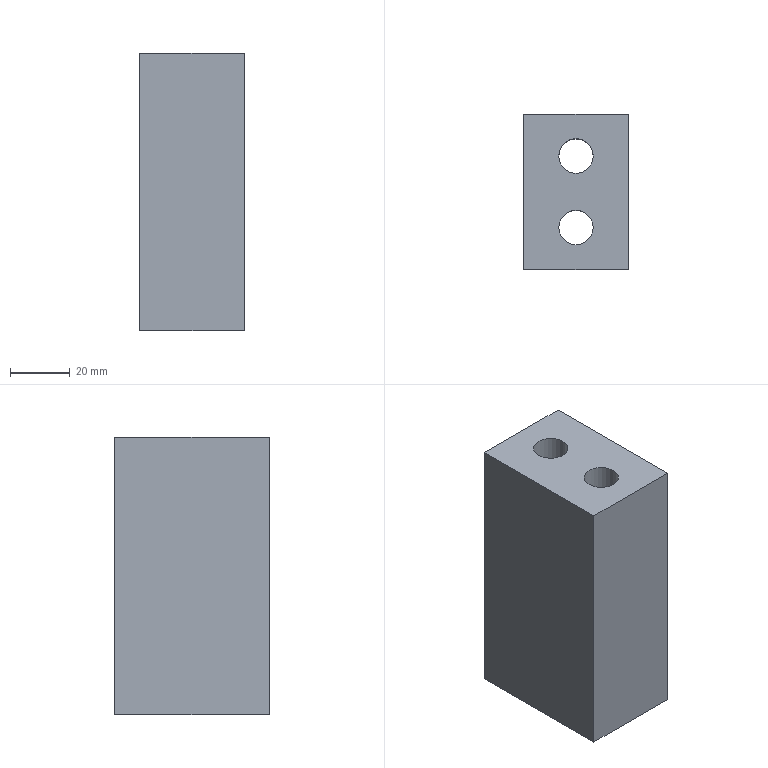Part | NX | features solid 2 | 1 solid | 12 faces | box 35 x 52 x 93 mm | volume 130929 mm3 | plane 8 | cylinder 4 | commonest cylinder face diameters 11.507 x2 18.008 x2
STEP:
#1=CARTESIAN_POINT('',(1828.477,105.595,64.999));
#2=VERTEX_POINT('',#1);
#3=CARTESIAN_POINT('',(1793.477,105.595,64.999));
#4=VERTEX_POINT('',#3);
#5=CARTESIAN_POINT('',(1793.477,105.595,64.999));
#6=DIRECTION('',(1.,0.,-0.000000004));
#7=VECTOR('',#6,1000.);
#8=LINE('',#5,#7);
#9=EDGE_CURVE('',#2,#4,#8,.F.);
#10=ORIENTED_EDGE('',*,*,#9,.F.);
#11=CARTESIAN_POINT('',(1828.477,105.595,-28.001));
#12=VERTEX_POINT('',#11);
#13=CARTESIAN_POINT('',(1828.477,105.595,44.999));
#14=DIRECTION('',(0.000000004,0.,1.));
#15=VECTOR('',#14,1000.);
#16=LINE('',#13,#15);
#17=EDGE_CURVE('',#12,#2,#16,.T.);
#18=ORIENTED_EDGE('',*,*,#17,.F.);
#19=CARTESIAN_POINT('',(1793.477,105.595,-28.001));
#20=VERTEX_POINT('',#19);
#21=CARTESIAN_POINT('',(1793.477,105.595,-28.001));
#22=DIRECTION('',(-1.,0.,0.000000004));
#23=VECTOR('',#22,1000.);
#24=LINE('',#21,#23);
#25=EDGE_CURVE('',#12,#20,#24,.T.);
#26=ORIENTED_EDGE('',*,*,#25,.T.);
#27=CARTESIAN_POINT('',(1793.477,105.595,44.999));
#28=DIRECTION('',(0.000000004,0.,1.));
#29=VECTOR('',#28,1000.);
#30=LINE('',#27,#29);
#31=EDGE_CURVE('',#20,#4,#30,.T.);
#32=ORIENTED_EDGE('',*,*,#31,.T.);
#33=EDGE_LOOP('',(#10,#18,#26,#32));
#34=FACE_BOUND('',#33,.T.);
#35=CARTESIAN_POINT('',(1793.477,105.595,44.999));
#36=DIRECTION('',(0.,-1.,0.));
#37=DIRECTION('',(0.000000004,0.,1.));
#38=AXIS2_PLACEMENT_3D('',#35,#36,#37);
#39=PLANE('',#38);
#40=ADVANCED_FACE('',(#34),#39,.F.);
#41=CARTESIAN_POINT('',(1801.973,91.595,-28.001));
#42=VERTEX_POINT('',#41);
#43=CARTESIAN_POINT('',(1810.977,91.595,-28.001));
#44=DIRECTION('',(0.000000004,0.,1.));
#45=DIRECTION('',(-1.,0.,0.000000004));
#46=AXIS2_PLACEMENT_3D('',#43,#44,#45);
#47=CIRCLE('',#46,9.004);
#48=EDGE_CURVE('',#42,#42,#47,.F.);
#49=ORIENTED_EDGE('',*,*,#48,.F.);
#50=EDGE_LOOP('',(#49));
#51=FACE_BOUND('',#50,.T.);
#52=CARTESIAN_POINT('',(1801.973,67.595,-28.001));
#53=VERTEX_POINT('',#52);
#54=CARTESIAN_POINT('',(1810.977,67.595,-28.001));
#55=DIRECTION('',(0.000000004,0.,1.));
#56=DIRECTION('',(-1.,0.,0.000000004));
#57=AXIS2_PLACEMENT_3D('',#54,#55,#56);
#58=CIRCLE('',#57,9.004);
#59=EDGE_CURVE('',#53,#53,#58,.F.);
#60=ORIENTED_EDGE('',*,*,#59,.F.);
#61=EDGE_LOOP('',(#60));
#62=FACE_BOUND('',#61,.T.);
#63=CARTESIAN_POINT('',(1793.477,53.595,-28.001));
#64=VERTEX_POINT('',#63);
#65=CARTESIAN_POINT('',(1793.477,-114.905,-28.001));
#66=DIRECTION('',(0.,1.,0.));
#67=VECTOR('',#66,1000.);
#68=LINE('',#65,#67);
#69=EDGE_CURVE('',#64,#20,#68,.T.);
#70=ORIENTED_EDGE('',*,*,#69,.T.);
#71=ORIENTED_EDGE('',*,*,#25,.F.);
#72=CARTESIAN_POINT('',(1828.477,53.595,-28.001));
#73=VERTEX_POINT('',#72);
#74=CARTESIAN_POINT('',(1828.477,-114.905,-28.001));
#75=DIRECTION('',(0.,1.,0.));
#76=VECTOR('',#75,1000.);
#77=LINE('',#74,#76);
#78=EDGE_CURVE('',#73,#12,#77,.T.);
#79=ORIENTED_EDGE('',*,*,#78,.F.);
#80=CARTESIAN_POINT('',(1793.477,53.595,-28.001));
#81=DIRECTION('',(-1.,0.,0.000000004));
#82=VECTOR('',#81,1000.);
#83=LINE('',#80,#82);
#84=EDGE_CURVE('',#73,#64,#83,.T.);
#85=ORIENTED_EDGE('',*,*,#84,.T.);
#86=EDGE_LOOP('',(#70,#71,#79,#85));
#87=FACE_BOUND('',#86,.T.);
#88=CARTESIAN_POINT('',(1793.477,-114.905,-28.001));
#89=DIRECTION('',(0.000000004,0.,1.));
#90=DIRECTION('',(0.,1.,0.));
#91=AXIS2_PLACEMENT_3D('',#88,#89,#90);
#92=PLANE('',#91);
#93=ADVANCED_FACE('',(#51,#62,#87),#92,.F.);
#94=CARTESIAN_POINT('',(1805.224,91.595,64.999));
#95=VERTEX_POINT('',#94);
#96=CARTESIAN_POINT('',(1810.977,91.595,64.999));
#97=DIRECTION('',(0.000000004,0.,1.));
#98=DIRECTION('',(-1.,0.,0.000000004));
#99=AXIS2_PLACEMENT_3D('',#96,#97,#98);
#100=CIRCLE('',#99,5.753);
#101=EDGE_CURVE('',#95,#95,#100,.T.);
#102=ORIENTED_EDGE('',*,*,#101,.F.);
#103=EDGE_LOOP('',(#102));
#104=FACE_BOUND('',#103,.T.);
#105=CARTESIAN_POINT('',(1805.224,67.595,64.999));
#106=VERTEX_POINT('',#105);
#107=CARTESIAN_POINT('',(1810.977,67.595,64.999));
#108=DIRECTION('',(0.000000004,0.,1.));
#109=DIRECTION('',(-1.,0.,0.000000004));
#110=AXIS2_PLACEMENT_3D('',#107,#108,#109);
#111=CIRCLE('',#110,5.753);
#112=EDGE_CURVE('',#106,#106,#111,.T.);
#113=ORIENTED_EDGE('',*,*,#112,.F.);
#114=EDGE_LOOP('',(#113));
#115=FACE_BOUND('',#114,.T.);
#116=CARTESIAN_POINT('',(1828.477,53.595,64.999));
#117=VERTEX_POINT('',#116);
#118=CARTESIAN_POINT('',(1828.477,-114.905,64.999));
#119=DIRECTION('',(0.,1.,0.));
#120=VECTOR('',#119,1000.);
#121=LINE('',#118,#120);
#122=EDGE_CURVE('',#2,#117,#121,.F.);
#123=ORIENTED_EDGE('',*,*,#122,.F.);
#124=ORIENTED_EDGE('',*,*,#9,.T.);
#125=CARTESIAN_POINT('',(1793.477,53.595,64.999));
#126=VERTEX_POINT('',#125);
#127=CARTESIAN_POINT('',(1793.477,-114.905,64.999));
#128=DIRECTION('',(0.,-1.,0.));
#129=VECTOR('',#128,1000.);
#130=LINE('',#127,#129);
#131=EDGE_CURVE('',#4,#126,#130,.T.);
#132=ORIENTED_EDGE('',*,*,#131,.T.);
#133=CARTESIAN_POINT('',(1793.477,53.595,64.999));
#134=DIRECTION('',(-1.,0.,0.000000004));
#135=VECTOR('',#134,1000.);
#136=LINE('',#133,#135);
#137=EDGE_CURVE('',#117,#126,#136,.T.);
#138=ORIENTED_EDGE('',*,*,#137,.F.);
#139=EDGE_LOOP('',(#123,#124,#132,#138));
#140=FACE_BOUND('',#139,.T.);
#141=CARTESIAN_POINT('',(1793.477,-114.905,64.999));
#142=DIRECTION('',(-0.000000004,0.,-1.));
#143=DIRECTION('',(0.,-1.,0.));
#144=AXIS2_PLACEMENT_3D('',#141,#142,#143);
#145=PLANE('',#144);
#146=ADVANCED_FACE('',(#104,#115,#140),#145,.F.);
#147=ORIENTED_EDGE('',*,*,#131,.F.);
#148=ORIENTED_EDGE('',*,*,#31,.F.);
#149=ORIENTED_EDGE('',*,*,#69,.F.);
#150=CARTESIAN_POINT('',(1793.477,53.595,44.999));
#151=DIRECTION('',(-0.000000004,0.,-1.));
#152=VECTOR('',#151,1000.);
#153=LINE('',#150,#152);
#154=EDGE_CURVE('',#126,#64,#153,.T.);
#155=ORIENTED_EDGE('',*,*,#154,.F.);
#156=EDGE_LOOP('',(#147,#148,#149,#155));
#157=FACE_BOUND('',#156,.T.);
#158=CARTESIAN_POINT('',(1793.477,-114.905,44.999));
#159=DIRECTION('',(1.,0.,-0.000000004));
#160=DIRECTION('',(0.000000004,0.,1.));
#161=AXIS2_PLACEMENT_3D('',#158,#159,#160);
#162=PLANE('',#161);
#163=ADVANCED_FACE('',(#157),#162,.F.);
#164=CARTESIAN_POINT('',(1828.477,53.595,44.999));
#165=DIRECTION('',(-0.000000004,0.,-1.));
#166=VECTOR('',#165,1000.);
#167=LINE('',#164,#166);
#168=EDGE_CURVE('',#117,#73,#167,.T.);
#169=ORIENTED_EDGE('',*,*,#168,.T.);
#170=ORIENTED_EDGE('',*,*,#78,.T.);
#171=ORIENTED_EDGE('',*,*,#17,.T.);
#172=ORIENTED_EDGE('',*,*,#122,.T.);
#173=EDGE_LOOP('',(#169,#170,#171,#172));
#174=FACE_BOUND('',#173,.T.);
#175=CARTESIAN_POINT('',(1828.477,-114.905,44.999));
#176=DIRECTION('',(1.,0.,-0.000000004));
#177=DIRECTION('',(0.000000004,0.,1.));
#178=AXIS2_PLACEMENT_3D('',#175,#176,#177);
#179=PLANE('',#178);
#180=ADVANCED_FACE('',(#174),#179,.T.);
#181=ORIENTED_EDGE('',*,*,#168,.F.);
#182=ORIENTED_EDGE('',*,*,#137,.T.);
#183=ORIENTED_EDGE('',*,*,#154,.T.);
#184=ORIENTED_EDGE('',*,*,#84,.F.);
#185=EDGE_LOOP('',(#181,#182,#183,#184));
#186=FACE_BOUND('',#185,.T.);
#187=CARTESIAN_POINT('',(1810.977,53.595,33.499));
#188=DIRECTION('',(0.,1.,0.));
#189=DIRECTION('',(1.,0.,0.));
#190=AXIS2_PLACEMENT_3D('',#187,#188,#189);
#191=PLANE('',#190);
#192=ADVANCED_FACE('',(#186),#191,.F.);
#193=CARTESIAN_POINT('',(1810.977,58.591,34.999));
#194=VERTEX_POINT('',#193);
#195=CARTESIAN_POINT('',(1810.977,67.595,34.999));
#196=DIRECTION('',(0.000000004,0.,1.));
#197=DIRECTION('',(0.,-1.,0.));
#198=AXIS2_PLACEMENT_3D('',#195,#196,#197);
#199=CIRCLE('',#198,9.004);
#200=EDGE_CURVE('',#194,#194,#199,.F.);
#201=ORIENTED_EDGE('',*,*,#200,.F.);
#202=EDGE_LOOP('',(#201));
#203=FACE_BOUND('',#202,.T.);
#204=ORIENTED_EDGE('',*,*,#59,.T.);
#205=EDGE_LOOP('',(#204));
#206=FACE_BOUND('',#205,.T.);
#207=CARTESIAN_POINT('',(1810.977,67.595,34.999));
#208=DIRECTION('',(-0.000000004,0.,-1.));
#209=DIRECTION('',(-1.,0.,0.000000004));
#210=AXIS2_PLACEMENT_3D('',#207,#208,#209);
#211=CYLINDRICAL_SURFACE('',#210,9.004);
#212=ADVANCED_FACE('',(#203,#206),#211,.F.);
#213=CARTESIAN_POINT('',(1805.224,67.595,34.999));
#214=VERTEX_POINT('',#213);
#215=CARTESIAN_POINT('',(1810.977,67.595,34.999));
#216=DIRECTION('',(0.000000004,0.,1.));
#217=DIRECTION('',(-1.,0.,0.000000004));
#218=AXIS2_PLACEMENT_3D('',#215,#216,#217);
#219=CIRCLE('',#218,5.753);
#220=EDGE_CURVE('',#214,#214,#219,.T.);
#221=ORIENTED_EDGE('',*,*,#220,.F.);
#222=EDGE_LOOP('',(#221));
#223=FACE_BOUND('',#222,.T.);
#224=ORIENTED_EDGE('',*,*,#112,.T.);
#225=EDGE_LOOP('',(#224));
#226=FACE_BOUND('',#225,.T.);
#227=CARTESIAN_POINT('',(1810.977,67.595,65.999));
#228=DIRECTION('',(-0.000000004,0.,-1.));
#229=DIRECTION('',(-1.,0.,0.000000004));
#230=AXIS2_PLACEMENT_3D('',#227,#228,#229);
#231=CYLINDRICAL_SURFACE('',#230,5.753);
#232=ADVANCED_FACE('',(#223,#226),#231,.F.);
#233=ORIENTED_EDGE('',*,*,#220,.T.);
#234=EDGE_LOOP('',(#233));
#235=FACE_BOUND('',#234,.T.);
#236=ORIENTED_EDGE('',*,*,#200,.T.);
#237=EDGE_LOOP('',(#236));
#238=FACE_BOUND('',#237,.T.);
#239=CARTESIAN_POINT('',(1810.977,67.595,34.999));
#240=DIRECTION('',(-0.000000004,0.,-1.));
#241=DIRECTION('',(-1.,0.,0.000000004));
#242=AXIS2_PLACEMENT_3D('',#239,#240,#241);
#243=PLANE('',#242);
#244=ADVANCED_FACE('',(#235,#238),#243,.T.);
#245=CARTESIAN_POINT('',(1810.977,82.591,34.999));
#246=VERTEX_POINT('',#245);
#247=CARTESIAN_POINT('',(1810.977,91.595,34.999));
#248=DIRECTION('',(0.000000004,0.,1.));
#249=DIRECTION('',(0.,-1.,0.));
#250=AXIS2_PLACEMENT_3D('',#247,#248,#249);
#251=CIRCLE('',#250,9.004);
#252=EDGE_CURVE('',#246,#246,#251,.F.);
#253=ORIENTED_EDGE('',*,*,#252,.F.);
#254=EDGE_LOOP('',(#253));
#255=FACE_BOUND('',#254,.T.);
#256=ORIENTED_EDGE('',*,*,#48,.T.);
#257=EDGE_LOOP('',(#256));
#258=FACE_BOUND('',#257,.T.);
#259=CARTESIAN_POINT('',(1810.977,91.595,34.999));
#260=DIRECTION('',(-0.000000004,0.,-1.));
#261=DIRECTION('',(-1.,0.,0.000000004));
#262=AXIS2_PLACEMENT_3D('',#259,#260,#261);
#263=CYLINDRICAL_SURFACE('',#262,9.004);
#264=ADVANCED_FACE('',(#255,#258),#263,.F.);
#265=CARTESIAN_POINT('',(1805.224,91.595,34.999));
#266=VERTEX_POINT('',#265);
#267=CARTESIAN_POINT('',(1810.977,91.595,34.999));
#268=DIRECTION('',(0.000000004,0.,1.));
#269=DIRECTION('',(-1.,0.,0.000000004));
#270=AXIS2_PLACEMENT_3D('',#267,#268,#269);
#271=CIRCLE('',#270,5.753);
#272=EDGE_CURVE('',#266,#266,#271,.T.);
#273=ORIENTED_EDGE('',*,*,#272,.F.);
#274=EDGE_LOOP('',(#273));
#275=FACE_BOUND('',#274,.T.);
#276=ORIENTED_EDGE('',*,*,#101,.T.);
#277=EDGE_LOOP('',(#276));
#278=FACE_BOUND('',#277,.T.);
#279=CARTESIAN_POINT('',(1810.977,91.595,65.999));
#280=DIRECTION('',(-0.000000004,0.,-1.));
#281=DIRECTION('',(-1.,0.,0.000000004));
#282=AXIS2_PLACEMENT_3D('',#279,#280,#281);
#283=CYLINDRICAL_SURFACE('',#282,5.753);
#284=ADVANCED_FACE('',(#275,#278),#283,.F.);
#285=ORIENTED_EDGE('',*,*,#272,.T.);
#286=EDGE_LOOP('',(#285));
#287=FACE_BOUND('',#286,.T.);
#288=ORIENTED_EDGE('',*,*,#252,.T.);
#289=EDGE_LOOP('',(#288));
#290=FACE_BOUND('',#289,.T.);
#291=CARTESIAN_POINT('',(1810.977,91.595,34.999));
#292=DIRECTION('',(-0.000000004,0.,-1.));
#293=DIRECTION('',(-1.,0.,0.000000004));
#294=AXIS2_PLACEMENT_3D('',#291,#292,#293);
#295=PLANE('',#294);
#296=ADVANCED_FACE('',(#287,#290),#295,.T.);
#297=CLOSED_SHELL('',(#40,#93,#146,#163,#180,#192,#212,#232,#244,#264,#284,#296));
#298=MANIFOLD_SOLID_BREP('',#297);
#299=(LENGTH_UNIT()NAMED_UNIT(*)SI_UNIT(.MILLI.,.METRE.));
#300=UNCERTAINTY_MEASURE_WITH_UNIT(LENGTH_MEASURE(0.00001),#299,'','');
#301=(NAMED_UNIT(*)PLANE_ANGLE_UNIT()SI_UNIT($,.RADIAN.));
#302=(NAMED_UNIT(*)SI_UNIT($,.STERADIAN.)SOLID_ANGLE_UNIT());
#303=(GEOMETRIC_REPRESENTATION_CONTEXT(3)GLOBAL_UNCERTAINTY_ASSIGNED_CONTEXT((#300))GLOBAL_UNIT_ASSIGNED_CONTEXT((#299,#301,#302))REPRESENTATION_CONTEXT('',''));
#304=ADVANCED_BREP_SHAPE_REPRESENTATION('',(#298),#303);